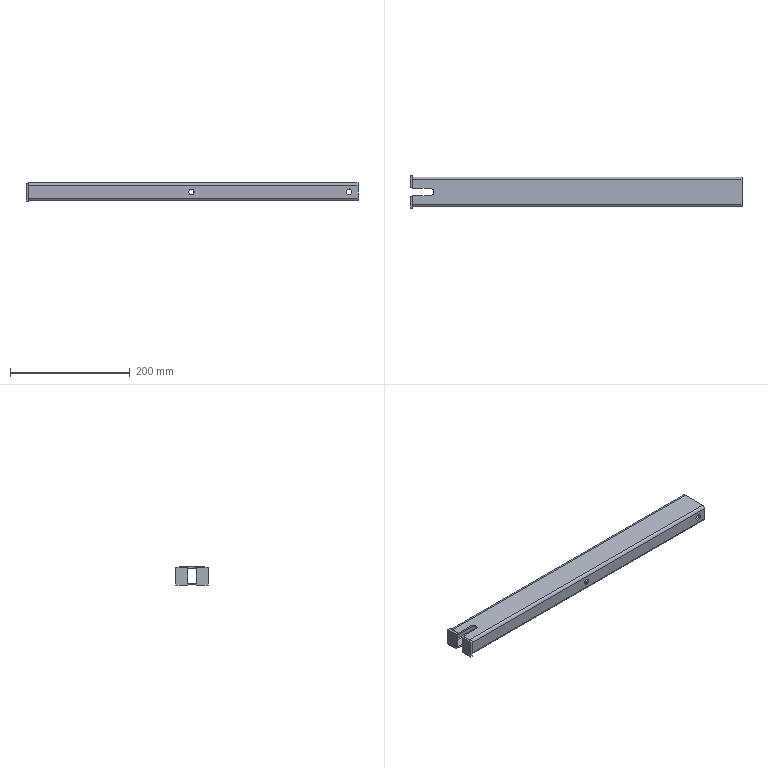Part | SolidWorks | features Cut 2, ICE 2, MirrorSolid 1, WeldMemberFeat 1, WeldmentFeature 1 | 3 solids | 47 faces | box 554 x 54 x 30.061 mm | volume 237150 mm3 | plane 27 | cylinder 20 | commonest cylinder face diameters 9 x8 3 x4 10 x4 12 x4
STEP:
#1=CARTESIAN_POINT('',(39.789,-25.,-4.5));
#2=VERTEX_POINT('',#1);
#3=CARTESIAN_POINT('',(39.789,-25.,4.5));
#4=VERTEX_POINT('',#3);
#5=CARTESIAN_POINT('',(39.789,-25.,0.));
#6=DIRECTION('',(0.,1.,0.));
#7=DIRECTION('',(0.,0.,1.));
#8=AXIS2_PLACEMENT_3D('',#5,#6,#7);
#9=CIRCLE('',#8,4.5);
#10=EDGE_CURVE('',#2,#4,#9,.T.);
#11=ORIENTED_EDGE('',*,*,#10,.F.);
#12=CARTESIAN_POINT('',(39.789,-22.,-4.5));
#13=VERTEX_POINT('',#12);
#14=CARTESIAN_POINT('',(39.789,-25.,-4.5));
#15=DIRECTION('',(0.,1.,0.));
#16=VECTOR('',#15,1000.);
#17=LINE('',#14,#16);
#18=EDGE_CURVE('',#2,#13,#17,.T.);
#19=ORIENTED_EDGE('',*,*,#18,.T.);
#20=CARTESIAN_POINT('',(39.789,-22.,4.5));
#21=VERTEX_POINT('',#20);
#22=CARTESIAN_POINT('',(39.789,-22.,0.));
#23=DIRECTION('',(0.,1.,0.));
#24=DIRECTION('',(0.,0.,1.));
#25=AXIS2_PLACEMENT_3D('',#22,#23,#24);
#26=CIRCLE('',#25,4.5);
#27=EDGE_CURVE('',#13,#21,#26,.T.);
#28=ORIENTED_EDGE('',*,*,#27,.T.);
#29=CARTESIAN_POINT('',(39.789,-25.,4.5));
#30=DIRECTION('',(0.,1.,0.));
#31=VECTOR('',#30,1000.);
#32=LINE('',#29,#31);
#33=EDGE_CURVE('',#4,#21,#32,.T.);
#34=ORIENTED_EDGE('',*,*,#33,.F.);
#35=EDGE_LOOP('',(#11,#19,#28,#34));
#36=FACE_OUTER_BOUND('',#35,.T.);
#37=CARTESIAN_POINT('',(39.789,-25.,0.));
#38=DIRECTION('',(0.,1.,0.));
#39=DIRECTION('',(0.,0.,1.));
#40=AXIS2_PLACEMENT_3D('',#37,#38,#39);
#41=CYLINDRICAL_SURFACE('',#40,4.5);
#42=ADVANCED_FACE('',(#36),#41,.F.);
#43=CARTESIAN_POINT('',(39.789,22.,4.5));
#44=VERTEX_POINT('',#43);
#45=CARTESIAN_POINT('',(39.789,22.,-4.5));
#46=VERTEX_POINT('',#45);
#47=CARTESIAN_POINT('',(39.789,22.,0.));
#48=DIRECTION('',(0.,-1.,0.));
#49=DIRECTION('',(0.,0.,-1.));
#50=AXIS2_PLACEMENT_3D('',#47,#48,#49);
#51=CIRCLE('',#50,4.5);
#52=EDGE_CURVE('',#44,#46,#51,.T.);
#53=ORIENTED_EDGE('',*,*,#52,.T.);
#54=CARTESIAN_POINT('',(39.789,25.,-4.5));
#55=VERTEX_POINT('',#54);
#56=CARTESIAN_POINT('',(39.789,-25.,-4.5));
#57=DIRECTION('',(0.,1.,0.));
#58=VECTOR('',#57,1000.);
#59=LINE('',#56,#58);
#60=EDGE_CURVE('',#46,#55,#59,.T.);
#61=ORIENTED_EDGE('',*,*,#60,.T.);
#62=CARTESIAN_POINT('',(39.789,25.,4.5));
#63=VERTEX_POINT('',#62);
#64=CARTESIAN_POINT('',(39.789,25.,0.));
#65=DIRECTION('',(0.,1.,0.));
#66=DIRECTION('',(0.,0.,1.));
#67=AXIS2_PLACEMENT_3D('',#64,#65,#66);
#68=CIRCLE('',#67,4.5);
#69=EDGE_CURVE('',#55,#63,#68,.T.);
#70=ORIENTED_EDGE('',*,*,#69,.T.);
#71=CARTESIAN_POINT('',(39.789,-25.,4.5));
#72=DIRECTION('',(0.,1.,0.));
#73=VECTOR('',#72,1000.);
#74=LINE('',#71,#73);
#75=EDGE_CURVE('',#44,#63,#74,.T.);
#76=ORIENTED_EDGE('',*,*,#75,.F.);
#77=EDGE_LOOP('',(#53,#61,#70,#76));
#78=FACE_OUTER_BOUND('',#77,.T.);
#79=CARTESIAN_POINT('',(39.789,-25.,0.));
#80=DIRECTION('',(0.,1.,0.));
#81=DIRECTION('',(0.,0.,1.));
#82=AXIS2_PLACEMENT_3D('',#79,#80,#81);
#83=CYLINDRICAL_SURFACE('',#82,4.5);
#84=ADVANCED_FACE('',(#78),#83,.F.);
#85=CARTESIAN_POINT('',(302.789,-22.,-5.));
#86=VERTEX_POINT('',#85);
#87=CARTESIAN_POINT('',(302.789,-22.,5.));
#88=VERTEX_POINT('',#87);
#89=CARTESIAN_POINT('',(302.789,-22.,0.));
#90=DIRECTION('',(0.,1.,0.));
#91=DIRECTION('',(0.,0.,1.));
#92=AXIS2_PLACEMENT_3D('',#89,#90,#91);
#93=CIRCLE('',#92,5.);
#94=EDGE_CURVE('',#86,#88,#93,.T.);
#95=ORIENTED_EDGE('',*,*,#94,.T.);
#96=CARTESIAN_POINT('',(302.789,-25.,5.));
#97=VERTEX_POINT('',#96);
#98=CARTESIAN_POINT('',(302.789,25.,5.));
#99=DIRECTION('',(0.,-1.,0.));
#100=VECTOR('',#99,1000.);
#101=LINE('',#98,#100);
#102=EDGE_CURVE('',#88,#97,#101,.T.);
#103=ORIENTED_EDGE('',*,*,#102,.T.);
#104=CARTESIAN_POINT('',(302.789,-25.,-5.));
#105=VERTEX_POINT('',#104);
#106=CARTESIAN_POINT('',(302.789,-25.,0.));
#107=DIRECTION('',(0.,-1.,0.));
#108=DIRECTION('',(0.,0.,-1.));
#109=AXIS2_PLACEMENT_3D('',#106,#107,#108);
#110=CIRCLE('',#109,5.);
#111=EDGE_CURVE('',#97,#105,#110,.T.);
#112=ORIENTED_EDGE('',*,*,#111,.T.);
#113=CARTESIAN_POINT('',(302.789,25.,-5.));
#114=DIRECTION('',(0.,-1.,0.));
#115=VECTOR('',#114,1000.);
#116=LINE('',#113,#115);
#117=EDGE_CURVE('',#86,#105,#116,.T.);
#118=ORIENTED_EDGE('',*,*,#117,.F.);
#119=EDGE_LOOP('',(#95,#103,#112,#118));
#120=FACE_OUTER_BOUND('',#119,.T.);
#121=CARTESIAN_POINT('',(302.789,25.,0.));
#122=DIRECTION('',(0.,-1.,0.));
#123=DIRECTION('',(0.,0.,-1.));
#124=AXIS2_PLACEMENT_3D('',#121,#122,#123);
#125=CYLINDRICAL_SURFACE('',#124,5.);
#126=ADVANCED_FACE('',(#120),#125,.F.);
#127=CARTESIAN_POINT('',(302.789,25.,5.));
#128=VERTEX_POINT('',#127);
#129=CARTESIAN_POINT('',(302.789,25.,-5.));
#130=VERTEX_POINT('',#129);
#131=CARTESIAN_POINT('',(302.789,25.,0.));
#132=DIRECTION('',(0.,-1.,0.));
#133=DIRECTION('',(0.,0.,-1.));
#134=AXIS2_PLACEMENT_3D('',#131,#132,#133);
#135=CIRCLE('',#134,5.);
#136=EDGE_CURVE('',#128,#130,#135,.T.);
#137=ORIENTED_EDGE('',*,*,#136,.F.);
#138=CARTESIAN_POINT('',(302.789,22.,5.));
#139=VERTEX_POINT('',#138);
#140=CARTESIAN_POINT('',(302.789,25.,5.));
#141=DIRECTION('',(0.,-1.,0.));
#142=VECTOR('',#141,1000.);
#143=LINE('',#140,#142);
#144=EDGE_CURVE('',#128,#139,#143,.T.);
#145=ORIENTED_EDGE('',*,*,#144,.T.);
#146=CARTESIAN_POINT('',(302.789,22.,-5.));
#147=VERTEX_POINT('',#146);
#148=CARTESIAN_POINT('',(302.789,22.,0.));
#149=DIRECTION('',(0.,-1.,0.));
#150=DIRECTION('',(0.,0.,-1.));
#151=AXIS2_PLACEMENT_3D('',#148,#149,#150);
#152=CIRCLE('',#151,5.);
#153=EDGE_CURVE('',#139,#147,#152,.T.);
#154=ORIENTED_EDGE('',*,*,#153,.T.);
#155=CARTESIAN_POINT('',(302.789,25.,-5.));
#156=DIRECTION('',(0.,-1.,0.));
#157=VECTOR('',#156,1000.);
#158=LINE('',#155,#157);
#159=EDGE_CURVE('',#130,#147,#158,.T.);
#160=ORIENTED_EDGE('',*,*,#159,.F.);
#161=EDGE_LOOP('',(#137,#145,#154,#160));
#162=FACE_OUTER_BOUND('',#161,.T.);
#163=CARTESIAN_POINT('',(302.789,25.,0.));
#164=DIRECTION('',(0.,-1.,0.));
#165=DIRECTION('',(0.,0.,-1.));
#166=AXIS2_PLACEMENT_3D('',#163,#164,#165);
#167=CYLINDRICAL_SURFACE('',#166,5.);
#168=ADVANCED_FACE('',(#162),#167,.F.);
#169=CARTESIAN_POINT('',(-202.211,6.,12.));
#170=VERTEX_POINT('',#169);
#171=CARTESIAN_POINT('',(-196.211,0.,12.));
#172=VERTEX_POINT('',#171);
#173=CARTESIAN_POINT('',(-202.211,0.,12.));
#174=DIRECTION('',(0.,0.,-1.));
#175=DIRECTION('',(-1.,0.,0.));
#176=AXIS2_PLACEMENT_3D('',#173,#174,#175);
#177=CIRCLE('',#176,6.);
#178=EDGE_CURVE('',#170,#172,#177,.T.);
#179=ORIENTED_EDGE('',*,*,#178,.T.);
#180=CARTESIAN_POINT('',(-196.211,0.,15.));
#181=VERTEX_POINT('',#180);
#182=CARTESIAN_POINT('',(-196.211,0.,-15.));
#183=DIRECTION('',(0.,0.,1.));
#184=VECTOR('',#183,1000.);
#185=LINE('',#182,#184);
#186=EDGE_CURVE('',#172,#181,#185,.T.);
#187=ORIENTED_EDGE('',*,*,#186,.T.);
#188=CARTESIAN_POINT('',(-202.211,6.,15.));
#189=VERTEX_POINT('',#188);
#190=CARTESIAN_POINT('',(-202.211,0.,15.));
#191=DIRECTION('',(0.,0.,1.));
#192=DIRECTION('',(1.,0.,0.));
#193=AXIS2_PLACEMENT_3D('',#190,#191,#192);
#194=CIRCLE('',#193,6.);
#195=EDGE_CURVE('',#181,#189,#194,.T.);
#196=ORIENTED_EDGE('',*,*,#195,.T.);
#197=CARTESIAN_POINT('',(-202.211,6.,-15.));
#198=DIRECTION('',(0.,0.,1.));
#199=VECTOR('',#198,1000.);
#200=LINE('',#197,#199);
#201=EDGE_CURVE('',#170,#189,#200,.T.);
#202=ORIENTED_EDGE('',*,*,#201,.F.);
#203=EDGE_LOOP('',(#179,#187,#196,#202));
#204=FACE_OUTER_BOUND('',#203,.T.);
#205=CARTESIAN_POINT('',(-202.211,0.,-15.));
#206=DIRECTION('',(0.,0.,1.));
#207=DIRECTION('',(1.,0.,0.));
#208=AXIS2_PLACEMENT_3D('',#205,#206,#207);
#209=CYLINDRICAL_SURFACE('',#208,6.);
#210=ADVANCED_FACE('',(#204),#209,.F.);
#211=CARTESIAN_POINT('',(-196.211,0.,-15.));
#212=VERTEX_POINT('',#211);
#213=CARTESIAN_POINT('',(-202.211,6.,-15.));
#214=VERTEX_POINT('',#213);
#215=CARTESIAN_POINT('',(-202.211,0.,-15.));
#216=DIRECTION('',(0.,0.,1.));
#217=DIRECTION('',(1.,0.,0.));
#218=AXIS2_PLACEMENT_3D('',#215,#216,#217);
#219=CIRCLE('',#218,6.);
#220=EDGE_CURVE('',#212,#214,#219,.T.);
#221=ORIENTED_EDGE('',*,*,#220,.F.);
#222=CARTESIAN_POINT('',(-196.211,0.,-12.));
#223=VERTEX_POINT('',#222);
#224=CARTESIAN_POINT('',(-196.211,0.,-15.));
#225=DIRECTION('',(0.,0.,1.));
#226=VECTOR('',#225,1000.);
#227=LINE('',#224,#226);
#228=EDGE_CURVE('',#212,#223,#227,.T.);
#229=ORIENTED_EDGE('',*,*,#228,.T.);
#230=CARTESIAN_POINT('',(-202.211,6.,-12.));
#231=VERTEX_POINT('',#230);
#232=CARTESIAN_POINT('',(-202.211,0.,-12.));
#233=DIRECTION('',(0.,0.,1.));
#234=DIRECTION('',(1.,0.,0.));
#235=AXIS2_PLACEMENT_3D('',#232,#233,#234);
#236=CIRCLE('',#235,6.);
#237=EDGE_CURVE('',#223,#231,#236,.T.);
#238=ORIENTED_EDGE('',*,*,#237,.T.);
#239=CARTESIAN_POINT('',(-202.211,6.,-15.));
#240=DIRECTION('',(0.,0.,1.));
#241=VECTOR('',#240,1000.);
#242=LINE('',#239,#241);
#243=EDGE_CURVE('',#214,#231,#242,.T.);
#244=ORIENTED_EDGE('',*,*,#243,.F.);
#245=EDGE_LOOP('',(#221,#229,#238,#244));
#246=FACE_OUTER_BOUND('',#245,.T.);
#247=CARTESIAN_POINT('',(-202.211,0.,-15.));
#248=DIRECTION('',(0.,0.,1.));
#249=DIRECTION('',(1.,0.,0.));
#250=AXIS2_PLACEMENT_3D('',#247,#248,#249);
#251=CYLINDRICAL_SURFACE('',#250,6.);
#252=ADVANCED_FACE('',(#246),#251,.F.);
#253=CARTESIAN_POINT('',(-232.211,6.,-15.));
#254=VERTEX_POINT('',#253);
#255=CARTESIAN_POINT('',(-232.211,20.5,-15.));
#256=VERTEX_POINT('',#255);
#257=CARTESIAN_POINT('',(-232.211,-20.5,-15.));
#258=DIRECTION('',(0.,1.,0.));
#259=VECTOR('',#258,1000.);
#260=LINE('',#257,#259);
#261=EDGE_CURVE('',#254,#256,#260,.T.);
#262=ORIENTED_EDGE('',*,*,#261,.F.);
#263=CARTESIAN_POINT('',(-232.211,6.,-12.));
#264=VERTEX_POINT('',#263);
#265=CARTESIAN_POINT('',(-232.211,6.,-15.));
#266=DIRECTION('',(0.,0.,1.));
#267=VECTOR('',#266,1000.);
#268=LINE('',#265,#267);
#269=EDGE_CURVE('',#254,#264,#268,.T.);
#270=ORIENTED_EDGE('',*,*,#269,.T.);
#271=CARTESIAN_POINT('',(-232.211,20.5,-12.));
#272=VERTEX_POINT('',#271);
#273=CARTESIAN_POINT('',(-232.211,-20.5,-12.));
#274=DIRECTION('',(0.,1.,0.));
#275=VECTOR('',#274,1000.);
#276=LINE('',#273,#275);
#277=EDGE_CURVE('',#264,#272,#276,.T.);
#278=ORIENTED_EDGE('',*,*,#277,.T.);
#279=CARTESIAN_POINT('',(-232.211,22.,-10.5));
#280=VERTEX_POINT('',#279);
#281=CARTESIAN_POINT('',(-232.211,20.5,-10.5));
#282=DIRECTION('',(1.,0.,0.));
#283=DIRECTION('',(0.,0.,-1.));
#284=AXIS2_PLACEMENT_3D('',#281,#282,#283);
#285=CIRCLE('',#284,1.5);
#286=EDGE_CURVE('',#272,#280,#285,.T.);
#287=ORIENTED_EDGE('',*,*,#286,.T.);
#288=CARTESIAN_POINT('',(-232.211,22.,10.5));
#289=VERTEX_POINT('',#288);
#290=CARTESIAN_POINT('',(-232.211,22.,10.5));
#291=DIRECTION('',(0.,0.,1.));
#292=VECTOR('',#291,1000.);
#293=LINE('',#290,#292);
#294=EDGE_CURVE('',#280,#289,#293,.T.);
#295=ORIENTED_EDGE('',*,*,#294,.T.);
#296=CARTESIAN_POINT('',(-232.211,20.5,12.));
#297=VERTEX_POINT('',#296);
#298=CARTESIAN_POINT('',(-232.211,20.5,10.5));
#299=DIRECTION('',(1.,0.,0.));
#300=DIRECTION('',(0.,0.,-1.));
#301=AXIS2_PLACEMENT_3D('',#298,#299,#300);
#302=CIRCLE('',#301,1.5);
#303=EDGE_CURVE('',#289,#297,#302,.T.);
#304=ORIENTED_EDGE('',*,*,#303,.T.);
#305=CARTESIAN_POINT('',(-232.211,6.,12.));
#306=VERTEX_POINT('',#305);
#307=CARTESIAN_POINT('',(-232.211,20.5,12.));
#308=DIRECTION('',(0.,-1.,0.));
#309=VECTOR('',#308,1000.);
#310=LINE('',#307,#309);
#311=EDGE_CURVE('',#297,#306,#310,.T.);
#312=ORIENTED_EDGE('',*,*,#311,.T.);
#313=CARTESIAN_POINT('',(-232.211,6.,15.));
#314=VERTEX_POINT('',#313);
#315=CARTESIAN_POINT('',(-232.211,6.,10.5));
#316=DIRECTION('',(0.,0.,1.));
#317=VECTOR('',#316,1000.);
#318=LINE('',#315,#317);
#319=EDGE_CURVE('',#306,#314,#318,.T.);
#320=ORIENTED_EDGE('',*,*,#319,.T.);
#321=CARTESIAN_POINT('',(-232.211,20.5,15.));
#322=VERTEX_POINT('',#321);
#323=CARTESIAN_POINT('',(-232.211,20.5,15.));
#324=DIRECTION('',(0.,-1.,0.));
#325=VECTOR('',#324,1000.);
#326=LINE('',#323,#325);
#327=EDGE_CURVE('',#322,#314,#326,.T.);
#328=ORIENTED_EDGE('',*,*,#327,.F.);
#329=CARTESIAN_POINT('',(-232.211,25.,10.5));
#330=VERTEX_POINT('',#329);
#331=CARTESIAN_POINT('',(-232.211,20.5,10.5));
#332=DIRECTION('',(1.,0.,0.));
#333=DIRECTION('',(0.,0.,-1.));
#334=AXIS2_PLACEMENT_3D('',#331,#332,#333);
#335=CIRCLE('',#334,4.5);
#336=EDGE_CURVE('',#330,#322,#335,.T.);
#337=ORIENTED_EDGE('',*,*,#336,.F.);
#338=CARTESIAN_POINT('',(-232.211,25.,-10.5));
#339=VERTEX_POINT('',#338);
#340=CARTESIAN_POINT('',(-232.211,25.,10.5));
#341=DIRECTION('',(0.,0.,1.));
#342=VECTOR('',#341,1000.);
#343=LINE('',#340,#342);
#344=EDGE_CURVE('',#339,#330,#343,.T.);
#345=ORIENTED_EDGE('',*,*,#344,.F.);
#346=CARTESIAN_POINT('',(-232.211,20.5,-10.5));
#347=DIRECTION('',(1.,0.,0.));
#348=DIRECTION('',(0.,0.,-1.));
#349=AXIS2_PLACEMENT_3D('',#346,#347,#348);
#350=CIRCLE('',#349,4.5);
#351=EDGE_CURVE('',#256,#339,#350,.T.);
#352=ORIENTED_EDGE('',*,*,#351,.F.);
#353=EDGE_LOOP('',(#262,#270,#278,#287,#295,#304,#312,#320,#328,#337,#345,#352));
#354=FACE_OUTER_BOUND('',#353,.T.);
#355=CARTESIAN_POINT('',(-232.211,20.5,10.5));
#356=DIRECTION('',(1.,0.,0.));
#357=DIRECTION('',(0.,0.,-1.));
#358=AXIS2_PLACEMENT_3D('',#355,#356,#357);
#359=PLANE('',#358);
#360=ADVANCED_FACE('',(#354),#359,.F.);
#361=ORIENTED_EDGE('',*,*,#336,.T.);
#362=CARTESIAN_POINT('',(317.789,20.5,15.));
#363=VERTEX_POINT('',#362);
#364=CARTESIAN_POINT('',(317.789,20.5,15.));
#365=DIRECTION('',(-1.,0.,0.));
#366=VECTOR('',#365,1000.);
#367=LINE('',#364,#366);
#368=EDGE_CURVE('',#363,#322,#367,.T.);
#369=ORIENTED_EDGE('',*,*,#368,.F.);
#370=CARTESIAN_POINT('',(317.789,25.,10.5));
#371=VERTEX_POINT('',#370);
#372=CARTESIAN_POINT('',(317.789,20.5,10.5));
#373=DIRECTION('',(1.,0.,0.));
#374=DIRECTION('',(0.,0.,-1.));
#375=AXIS2_PLACEMENT_3D('',#372,#373,#374);
#376=CIRCLE('',#375,4.5);
#377=EDGE_CURVE('',#371,#363,#376,.T.);
#378=ORIENTED_EDGE('',*,*,#377,.F.);
#379=CARTESIAN_POINT('',(317.789,25.,10.5));
#380=DIRECTION('',(-1.,0.,0.));
#381=VECTOR('',#380,1000.);
#382=LINE('',#379,#381);
#383=EDGE_CURVE('',#371,#330,#382,.T.);
#384=ORIENTED_EDGE('',*,*,#383,.T.);
#385=EDGE_LOOP('',(#361,#369,#378,#384));
#386=FACE_OUTER_BOUND('',#385,.T.);
#387=CARTESIAN_POINT('',(317.789,20.5,10.5));
#388=DIRECTION('',(-1.,0.,0.));
#389=DIRECTION('',(0.,0.,1.));
#390=AXIS2_PLACEMENT_3D('',#387,#388,#389);
#391=CYLINDRICAL_SURFACE('',#390,4.5);
#392=ADVANCED_FACE('',(#386),#391,.T.);
#393=ORIENTED_EDGE('',*,*,#327,.T.);
#394=CARTESIAN_POINT('',(-232.211,6.,15.));
#395=DIRECTION('',(-1.,0.,0.));
#396=VECTOR('',#395,1000.);
#397=LINE('',#394,#396);
#398=EDGE_CURVE('',#189,#314,#397,.T.);
#399=ORIENTED_EDGE('',*,*,#398,.F.);
#400=ORIENTED_EDGE('',*,*,#195,.F.);
#401=CARTESIAN_POINT('',(-202.211,-6.,15.));
#402=VERTEX_POINT('',#401);
#403=CARTESIAN_POINT('',(-202.211,0.,15.));
#404=DIRECTION('',(0.,0.,1.));
#405=DIRECTION('',(1.,0.,0.));
#406=AXIS2_PLACEMENT_3D('',#403,#404,#405);
#407=CIRCLE('',#406,6.);
#408=EDGE_CURVE('',#402,#181,#407,.T.);
#409=ORIENTED_EDGE('',*,*,#408,.F.);
#410=CARTESIAN_POINT('',(-232.211,-6.,15.));
#411=VERTEX_POINT('',#410);
#412=CARTESIAN_POINT('',(-232.211,-6.,15.));
#413=DIRECTION('',(1.,0.,0.));
#414=VECTOR('',#413,1000.);
#415=LINE('',#412,#414);
#416=EDGE_CURVE('',#411,#402,#415,.T.);
#417=ORIENTED_EDGE('',*,*,#416,.F.);
#418=CARTESIAN_POINT('',(-232.211,-20.5,15.));
#419=VERTEX_POINT('',#418);
#420=CARTESIAN_POINT('',(-232.211,20.5,15.));
#421=DIRECTION('',(0.,-1.,0.));
#422=VECTOR('',#421,1000.);
#423=LINE('',#420,#422);
#424=EDGE_CURVE('',#411,#419,#423,.T.);
#425=ORIENTED_EDGE('',*,*,#424,.T.);
#426=CARTESIAN_POINT('',(317.789,-20.5,15.));
#427=VERTEX_POINT('',#426);
#428=CARTESIAN_POINT('',(317.789,-20.5,15.));
#429=DIRECTION('',(-1.,0.,0.));
#430=VECTOR('',#429,1000.);
#431=LINE('',#428,#430);
#432=EDGE_CURVE('',#427,#419,#431,.T.);
#433=ORIENTED_EDGE('',*,*,#432,.F.);
#434=CARTESIAN_POINT('',(317.789,20.5,15.));
#435=DIRECTION('',(0.,-1.,0.));
#436=VECTOR('',#435,1000.);
#437=LINE('',#434,#436);
#438=EDGE_CURVE('',#363,#427,#437,.T.);
#439=ORIENTED_EDGE('',*,*,#438,.F.);
#440=ORIENTED_EDGE('',*,*,#368,.T.);
#441=EDGE_LOOP('',(#393,#399,#400,#409,#417,#425,#433,#439,#440));
#442=FACE_OUTER_BOUND('',#441,.T.);
#443=CARTESIAN_POINT('',(317.789,20.5,15.));
#444=DIRECTION('',(0.,0.,-1.));
#445=DIRECTION('',(-1.,0.,0.));
#446=AXIS2_PLACEMENT_3D('',#443,#444,#445);
#447=PLANE('',#446);
#448=ADVANCED_FACE('',(#442),#447,.F.);
#449=CARTESIAN_POINT('',(-232.211,-25.,10.5));
#450=VERTEX_POINT('',#449);
#451=CARTESIAN_POINT('',(-232.211,-20.5,10.5));
#452=DIRECTION('',(1.,0.,0.));
#453=DIRECTION('',(0.,0.,-1.));
#454=AXIS2_PLACEMENT_3D('',#451,#452,#453);
#455=CIRCLE('',#454,4.5);
#456=EDGE_CURVE('',#419,#450,#455,.T.);
#457=ORIENTED_EDGE('',*,*,#456,.T.);
#458=CARTESIAN_POINT('',(317.789,-25.,10.5));
#459=VERTEX_POINT('',#458);
#460=CARTESIAN_POINT('',(317.789,-25.,10.5));
#461=DIRECTION('',(-1.,0.,0.));
#462=VECTOR('',#461,1000.);
#463=LINE('',#460,#462);
#464=EDGE_CURVE('',#459,#450,#463,.T.);
#465=ORIENTED_EDGE('',*,*,#464,.F.);
#466=CARTESIAN_POINT('',(317.789,-20.5,10.5));
#467=DIRECTION('',(1.,0.,0.));
#468=DIRECTION('',(0.,0.,-1.));
#469=AXIS2_PLACEMENT_3D('',#466,#467,#468);
#470=CIRCLE('',#469,4.5);
#471=EDGE_CURVE('',#427,#459,#470,.T.);
#472=ORIENTED_EDGE('',*,*,#471,.F.);
#473=ORIENTED_EDGE('',*,*,#432,.T.);
#474=EDGE_LOOP('',(#457,#465,#472,#473));
#475=FACE_OUTER_BOUND('',#474,.T.);
#476=CARTESIAN_POINT('',(317.789,-20.5,10.5));
#477=DIRECTION('',(-1.,0.,0.));
#478=DIRECTION('',(0.,0.,1.));
#479=AXIS2_PLACEMENT_3D('',#476,#477,#478);
#480=CYLINDRICAL_SURFACE('',#479,4.5);
#481=ADVANCED_FACE('',(#475),#480,.T.);
#482=CARTESIAN_POINT('',(39.789,-25.,0.));
#483=DIRECTION('',(0.,1.,0.));
#484=DIRECTION('',(0.,0.,1.));
#485=AXIS2_PLACEMENT_3D('',#482,#483,#484);
#486=CIRCLE('',#485,4.5);
#487=EDGE_CURVE('',#4,#2,#486,.T.);
#488=ORIENTED_EDGE('',*,*,#487,.T.);
#489=ORIENTED_EDGE('',*,*,#10,.T.);
#490=EDGE_LOOP('',(#488,#489));
#491=FACE_BOUND('',#490,.T.);
#492=CARTESIAN_POINT('',(302.789,-25.,0.));
#493=DIRECTION('',(0.,-1.,0.));
#494=DIRECTION('',(0.,0.,-1.));
#495=AXIS2_PLACEMENT_3D('',#492,#493,#494);
#496=CIRCLE('',#495,5.);
#497=EDGE_CURVE('',#105,#97,#496,.T.);
#498=ORIENTED_EDGE('',*,*,#497,.F.);
#499=ORIENTED_EDGE('',*,*,#111,.F.);
#500=EDGE_LOOP('',(#498,#499));
#501=FACE_BOUND('',#500,.T.);
#502=CARTESIAN_POINT('',(-232.211,-25.,-10.5));
#503=VERTEX_POINT('',#502);
#504=CARTESIAN_POINT('',(-232.211,-25.,-10.5));
#505=DIRECTION('',(0.,0.,-1.));
#506=VECTOR('',#505,1000.);
#507=LINE('',#504,#506);
#508=EDGE_CURVE('',#450,#503,#507,.T.);
#509=ORIENTED_EDGE('',*,*,#508,.T.);
#510=CARTESIAN_POINT('',(317.789,-25.,-10.5));
#511=VERTEX_POINT('',#510);
#512=CARTESIAN_POINT('',(317.789,-25.,-10.5));
#513=DIRECTION('',(-1.,0.,0.));
#514=VECTOR('',#513,1000.);
#515=LINE('',#512,#514);
#516=EDGE_CURVE('',#511,#503,#515,.T.);
#517=ORIENTED_EDGE('',*,*,#516,.F.);
#518=CARTESIAN_POINT('',(317.789,-25.,-10.5));
#519=DIRECTION('',(0.,0.,-1.));
#520=VECTOR('',#519,1000.);
#521=LINE('',#518,#520);
#522=EDGE_CURVE('',#459,#511,#521,.T.);
#523=ORIENTED_EDGE('',*,*,#522,.F.);
#524=ORIENTED_EDGE('',*,*,#464,.T.);
#525=EDGE_LOOP('',(#509,#517,#523,#524));
#526=FACE_OUTER_BOUND('',#525,.T.);
#527=CARTESIAN_POINT('',(317.789,-25.,-10.5));
#528=DIRECTION('',(0.,1.,0.));
#529=DIRECTION('',(0.,0.,1.));
#530=AXIS2_PLACEMENT_3D('',#527,#528,#529);
#531=PLANE('',#530);
#532=ADVANCED_FACE('',(#491,#501,#526),#531,.F.);
#533=CARTESIAN_POINT('',(-232.211,-20.5,-15.));
#534=VERTEX_POINT('',#533);
#535=CARTESIAN_POINT('',(-232.211,-20.5,-10.5));
#536=DIRECTION('',(1.,0.,0.));
#537=DIRECTION('',(0.,0.,-1.));
#538=AXIS2_PLACEMENT_3D('',#535,#536,#537);
#539=CIRCLE('',#538,4.5);
#540=EDGE_CURVE('',#503,#534,#539,.T.);
#541=ORIENTED_EDGE('',*,*,#540,.T.);
#542=CARTESIAN_POINT('',(317.789,-20.5,-15.));
#543=VERTEX_POINT('',#542);
#544=CARTESIAN_POINT('',(317.789,-20.5,-15.));
#545=DIRECTION('',(-1.,0.,0.));
#546=VECTOR('',#545,1000.);
#547=LINE('',#544,#546);
#548=EDGE_CURVE('',#543,#534,#547,.T.);
#549=ORIENTED_EDGE('',*,*,#548,.F.);
#550=CARTESIAN_POINT('',(317.789,-20.5,-10.5));
#551=DIRECTION('',(1.,0.,0.));
#552=DIRECTION('',(0.,0.,-1.));
#553=AXIS2_PLACEMENT_3D('',#550,#551,#552);
#554=CIRCLE('',#553,4.5);
#555=EDGE_CURVE('',#511,#543,#554,.T.);
#556=ORIENTED_EDGE('',*,*,#555,.F.);
#557=ORIENTED_EDGE('',*,*,#516,.T.);
#558=EDGE_LOOP('',(#541,#549,#556,#557));
#559=FACE_OUTER_BOUND('',#558,.T.);
#560=CARTESIAN_POINT('',(317.789,-20.5,-10.5));
#561=DIRECTION('',(-1.,0.,0.));
#562=DIRECTION('',(0.,0.,1.));
#563=AXIS2_PLACEMENT_3D('',#560,#561,#562);
#564=CYLINDRICAL_SURFACE('',#563,4.5);
#565=ADVANCED_FACE('',(#559),#564,.T.);
#566=CARTESIAN_POINT('',(-202.211,-6.,-15.));
#567=VERTEX_POINT('',#566);
#568=CARTESIAN_POINT('',(-202.211,0.,-15.));
#569=DIRECTION('',(0.,0.,1.));
#570=DIRECTION('',(1.,0.,0.));
#571=AXIS2_PLACEMENT_3D('',#568,#569,#570);
#572=CIRCLE('',#571,6.);
#573=EDGE_CURVE('',#567,#212,#572,.T.);
#574=ORIENTED_EDGE('',*,*,#573,.T.);
#575=ORIENTED_EDGE('',*,*,#220,.T.);
#576=CARTESIAN_POINT('',(-232.211,6.,-15.));
#577=DIRECTION('',(-1.,0.,0.));
#578=VECTOR('',#577,1000.);
#579=LINE('',#576,#578);
#580=EDGE_CURVE('',#214,#254,#579,.T.);
#581=ORIENTED_EDGE('',*,*,#580,.T.);
#582=ORIENTED_EDGE('',*,*,#261,.T.);
#583=CARTESIAN_POINT('',(317.789,20.5,-15.));
#584=VERTEX_POINT('',#583);
#585=CARTESIAN_POINT('',(317.789,20.5,-15.));
#586=DIRECTION('',(-1.,0.,0.));
#587=VECTOR('',#586,1000.);
#588=LINE('',#585,#587);
#589=EDGE_CURVE('',#584,#256,#588,.T.);
#590=ORIENTED_EDGE('',*,*,#589,.F.);
#591=CARTESIAN_POINT('',(317.789,-20.5,-15.));
#592=DIRECTION('',(0.,1.,0.));
#593=VECTOR('',#592,1000.);
#594=LINE('',#591,#593);
#595=EDGE_CURVE('',#543,#584,#594,.T.);
#596=ORIENTED_EDGE('',*,*,#595,.F.);
#597=ORIENTED_EDGE('',*,*,#548,.T.);
#598=CARTESIAN_POINT('',(-232.211,-6.,-15.));
#599=VERTEX_POINT('',#598);
#600=CARTESIAN_POINT('',(-232.211,-20.5,-15.));
#601=DIRECTION('',(0.,1.,0.));
#602=VECTOR('',#601,1000.);
#603=LINE('',#600,#602);
#604=EDGE_CURVE('',#534,#599,#603,.T.);
#605=ORIENTED_EDGE('',*,*,#604,.T.);
#606=CARTESIAN_POINT('',(-232.211,-6.,-15.));
#607=DIRECTION('',(1.,0.,0.));
#608=VECTOR('',#607,1000.);
#609=LINE('',#606,#608);
#610=EDGE_CURVE('',#599,#567,#609,.T.);
#611=ORIENTED_EDGE('',*,*,#610,.T.);
#612=EDGE_LOOP('',(#574,#575,#581,#582,#590,#596,#597,#605,#611));
#613=FACE_OUTER_BOUND('',#612,.T.);
#614=CARTESIAN_POINT('',(317.789,-20.5,-15.));
#615=DIRECTION('',(0.,0.,1.));
#616=DIRECTION('',(1.,0.,0.));
#617=AXIS2_PLACEMENT_3D('',#614,#615,#616);
#618=PLANE('',#617);
#619=ADVANCED_FACE('',(#613),#618,.F.);
#620=ORIENTED_EDGE('',*,*,#351,.T.);
#621=CARTESIAN_POINT('',(317.789,25.,-10.5));
#622=VERTEX_POINT('',#621);
#623=CARTESIAN_POINT('',(317.789,25.,-10.5));
#624=DIRECTION('',(-1.,0.,0.));
#625=VECTOR('',#624,1000.);
#626=LINE('',#623,#625);
#627=EDGE_CURVE('',#622,#339,#626,.T.);
#628=ORIENTED_EDGE('',*,*,#627,.F.);
#629=CARTESIAN_POINT('',(317.789,20.5,-10.5));
#630=DIRECTION('',(1.,0.,0.));
#631=DIRECTION('',(0.,0.,-1.));
#632=AXIS2_PLACEMENT_3D('',#629,#630,#631);
#633=CIRCLE('',#632,4.5);
#634=EDGE_CURVE('',#584,#622,#633,.T.);
#635=ORIENTED_EDGE('',*,*,#634,.F.);
#636=ORIENTED_EDGE('',*,*,#589,.T.);
#637=EDGE_LOOP('',(#620,#628,#635,#636));
#638=FACE_OUTER_BOUND('',#637,.T.);
#639=CARTESIAN_POINT('',(317.789,20.5,-10.5));
#640=DIRECTION('',(-1.,0.,0.));
#641=DIRECTION('',(0.,0.,1.));
#642=AXIS2_PLACEMENT_3D('',#639,#640,#641);
#643=CYLINDRICAL_SURFACE('',#642,4.5);
#644=ADVANCED_FACE('',(#638),#643,.T.);
#645=CARTESIAN_POINT('',(-232.211,-20.5,12.));
#646=VERTEX_POINT('',#645);
#647=CARTESIAN_POINT('',(-232.211,-22.,10.5));
#648=VERTEX_POINT('',#647);
#649=CARTESIAN_POINT('',(-232.211,-20.5,10.5));
#650=DIRECTION('',(1.,0.,0.));
#651=DIRECTION('',(0.,0.,-1.));
#652=AXIS2_PLACEMENT_3D('',#649,#650,#651);
#653=CIRCLE('',#652,1.5);
#654=EDGE_CURVE('',#646,#648,#653,.T.);
#655=ORIENTED_EDGE('',*,*,#654,.F.);
#656=CARTESIAN_POINT('',(317.789,-20.5,12.));
#657=VERTEX_POINT('',#656);
#658=CARTESIAN_POINT('',(317.789,-20.5,12.));
#659=DIRECTION('',(-1.,0.,0.));
#660=VECTOR('',#659,1000.);
#661=LINE('',#658,#660);
#662=EDGE_CURVE('',#657,#646,#661,.T.);
#663=ORIENTED_EDGE('',*,*,#662,.F.);
#664=CARTESIAN_POINT('',(317.789,-22.,10.5));
#665=VERTEX_POINT('',#664);
#666=CARTESIAN_POINT('',(317.789,-20.5,10.5));
#667=DIRECTION('',(1.,0.,0.));
#668=DIRECTION('',(0.,0.,-1.));
#669=AXIS2_PLACEMENT_3D('',#666,#667,#668);
#670=CIRCLE('',#669,1.5);
#671=EDGE_CURVE('',#657,#665,#670,.T.);
#672=ORIENTED_EDGE('',*,*,#671,.T.);
#673=CARTESIAN_POINT('',(317.789,-22.,10.5));
#674=DIRECTION('',(-1.,0.,0.));
#675=VECTOR('',#674,1000.);
#676=LINE('',#673,#675);
#677=EDGE_CURVE('',#665,#648,#676,.T.);
#678=ORIENTED_EDGE('',*,*,#677,.T.);
#679=EDGE_LOOP('',(#655,#663,#672,#678));
#680=FACE_OUTER_BOUND('',#679,.T.);
#681=CARTESIAN_POINT('',(317.789,-20.5,10.5));
#682=DIRECTION('',(-1.,0.,0.));
#683=DIRECTION('',(0.,0.,1.));
#684=AXIS2_PLACEMENT_3D('',#681,#682,#683);
#685=CYLINDRICAL_SURFACE('',#684,1.5);
#686=ADVANCED_FACE('',(#680),#685,.F.);
#687=CARTESIAN_POINT('',(317.789,6.,12.));
#688=DIRECTION('',(1.,0.,0.));
#689=VECTOR('',#688,1000.);
#690=LINE('',#687,#689);
#691=EDGE_CURVE('',#306,#170,#690,.T.);
#692=ORIENTED_EDGE('',*,*,#691,.F.);
#693=ORIENTED_EDGE('',*,*,#311,.F.);
#694=CARTESIAN_POINT('',(317.789,20.5,12.));
#695=VERTEX_POINT('',#694);
#696=CARTESIAN_POINT('',(317.789,20.5,12.));
#697=DIRECTION('',(-1.,0.,0.));
#698=VECTOR('',#697,1000.);
#699=LINE('',#696,#698);
#700=EDGE_CURVE('',#695,#297,#699,.T.);
#701=ORIENTED_EDGE('',*,*,#700,.F.);
#702=CARTESIAN_POINT('',(317.789,20.5,12.));
#703=DIRECTION('',(0.,-1.,0.));
#704=VECTOR('',#703,1000.);
#705=LINE('',#702,#704);
#706=EDGE_CURVE('',#695,#657,#705,.T.);
#707=ORIENTED_EDGE('',*,*,#706,.T.);
#708=ORIENTED_EDGE('',*,*,#662,.T.);
#709=CARTESIAN_POINT('',(-232.211,-6.,12.));
#710=VERTEX_POINT('',#709);
#711=CARTESIAN_POINT('',(-232.211,20.5,12.));
#712=DIRECTION('',(0.,-1.,0.));
#713=VECTOR('',#712,1000.);
#714=LINE('',#711,#713);
#715=EDGE_CURVE('',#710,#646,#714,.T.);
#716=ORIENTED_EDGE('',*,*,#715,.F.);
#717=CARTESIAN_POINT('',(-202.211,-6.,12.));
#718=VERTEX_POINT('',#717);
#719=CARTESIAN_POINT('',(317.789,-6.,12.));
#720=DIRECTION('',(-1.,0.,0.));
#721=VECTOR('',#720,1000.);
#722=LINE('',#719,#721);
#723=EDGE_CURVE('',#718,#710,#722,.T.);
#724=ORIENTED_EDGE('',*,*,#723,.F.);
#725=CARTESIAN_POINT('',(-202.211,0.,12.));
#726=DIRECTION('',(0.,0.,-1.));
#727=DIRECTION('',(-1.,0.,0.));
#728=AXIS2_PLACEMENT_3D('',#725,#726,#727);
#729=CIRCLE('',#728,6.);
#730=EDGE_CURVE('',#172,#718,#729,.T.);
#731=ORIENTED_EDGE('',*,*,#730,.F.);
#732=ORIENTED_EDGE('',*,*,#178,.F.);
#733=EDGE_LOOP('',(#692,#693,#701,#707,#708,#716,#724,#731,#732));
#734=FACE_OUTER_BOUND('',#733,.T.);
#735=CARTESIAN_POINT('',(317.789,20.5,12.));
#736=DIRECTION('',(0.,0.,-1.));
#737=DIRECTION('',(-1.,0.,0.));
#738=AXIS2_PLACEMENT_3D('',#735,#736,#737);
#739=PLANE('',#738);
#740=ADVANCED_FACE('',(#734),#739,.T.);
#741=ORIENTED_EDGE('',*,*,#303,.F.);
#742=CARTESIAN_POINT('',(317.789,22.,10.5));
#743=VERTEX_POINT('',#742);
#744=CARTESIAN_POINT('',(317.789,22.,10.5));
#745=DIRECTION('',(-1.,0.,0.));
#746=VECTOR('',#745,1000.);
#747=LINE('',#744,#746);
#748=EDGE_CURVE('',#743,#289,#747,.T.);
#749=ORIENTED_EDGE('',*,*,#748,.F.);
#750=CARTESIAN_POINT('',(317.789,20.5,10.5));
#751=DIRECTION('',(1.,0.,0.));
#752=DIRECTION('',(0.,0.,-1.));
#753=AXIS2_PLACEMENT_3D('',#750,#751,#752);
#754=CIRCLE('',#753,1.5);
#755=EDGE_CURVE('',#743,#695,#754,.T.);
#756=ORIENTED_EDGE('',*,*,#755,.T.);
#757=ORIENTED_EDGE('',*,*,#700,.T.);
#758=EDGE_LOOP('',(#741,#749,#756,#757));
#759=FACE_OUTER_BOUND('',#758,.T.);
#760=CARTESIAN_POINT('',(317.789,20.5,10.5));
#761=DIRECTION('',(-1.,0.,0.));
#762=DIRECTION('',(0.,0.,1.));
#763=AXIS2_PLACEMENT_3D('',#760,#761,#762);
#764=CYLINDRICAL_SURFACE('',#763,1.5);
#765=ADVANCED_FACE('',(#759),#764,.F.);
#766=ORIENTED_EDGE('',*,*,#52,.F.);
#767=CARTESIAN_POINT('',(39.789,22.,0.));
#768=DIRECTION('',(0.,-1.,0.));
#769=DIRECTION('',(0.,0.,-1.));
#770=AXIS2_PLACEMENT_3D('',#767,#768,#769);
#771=CIRCLE('',#770,4.5);
#772=EDGE_CURVE('',#46,#44,#771,.T.);
#773=ORIENTED_EDGE('',*,*,#772,.F.);
#774=EDGE_LOOP('',(#766,#773));
#775=FACE_BOUND('',#774,.T.);
#776=CARTESIAN_POINT('',(302.789,22.,0.));
#777=DIRECTION('',(0.,-1.,0.));
#778=DIRECTION('',(0.,0.,-1.));
#779=AXIS2_PLACEMENT_3D('',#776,#777,#778);
#780=CIRCLE('',#779,5.);
#781=EDGE_CURVE('',#147,#139,#780,.T.);
#782=ORIENTED_EDGE('',*,*,#781,.F.);
#783=ORIENTED_EDGE('',*,*,#153,.F.);
#784=EDGE_LOOP('',(#782,#783));
#785=FACE_BOUND('',#784,.T.);
#786=ORIENTED_EDGE('',*,*,#294,.F.);
#787=CARTESIAN_POINT('',(317.789,22.,-10.5));
#788=VERTEX_POINT('',#787);
#789=CARTESIAN_POINT('',(317.789,22.,-10.5));
#790=DIRECTION('',(-1.,0.,0.));
#791=VECTOR('',#790,1000.);
#792=LINE('',#789,#791);
#793=EDGE_CURVE('',#788,#280,#792,.T.);
#794=ORIENTED_EDGE('',*,*,#793,.F.);
#795=CARTESIAN_POINT('',(317.789,22.,10.5));
#796=DIRECTION('',(0.,0.,1.));
#797=VECTOR('',#796,1000.);
#798=LINE('',#795,#797);
#799=EDGE_CURVE('',#788,#743,#798,.T.);
#800=ORIENTED_EDGE('',*,*,#799,.T.);
#801=ORIENTED_EDGE('',*,*,#748,.T.);
#802=EDGE_LOOP('',(#786,#794,#800,#801));
#803=FACE_OUTER_BOUND('',#802,.T.);
#804=CARTESIAN_POINT('',(317.789,22.,10.5));
#805=DIRECTION('',(0.,-1.,0.));
#806=DIRECTION('',(0.,0.,-1.));
#807=AXIS2_PLACEMENT_3D('',#804,#805,#806);
#808=PLANE('',#807);
#809=ADVANCED_FACE('',(#775,#785,#803),#808,.T.);
#810=ORIENTED_EDGE('',*,*,#286,.F.);
#811=CARTESIAN_POINT('',(317.789,20.5,-12.));
#812=VERTEX_POINT('',#811);
#813=CARTESIAN_POINT('',(317.789,20.5,-12.));
#814=DIRECTION('',(-1.,0.,0.));
#815=VECTOR('',#814,1000.);
#816=LINE('',#813,#815);
#817=EDGE_CURVE('',#812,#272,#816,.T.);
#818=ORIENTED_EDGE('',*,*,#817,.F.);
#819=CARTESIAN_POINT('',(317.789,20.5,-10.5));
#820=DIRECTION('',(1.,0.,0.));
#821=DIRECTION('',(0.,0.,-1.));
#822=AXIS2_PLACEMENT_3D('',#819,#820,#821);
#823=CIRCLE('',#822,1.5);
#824=EDGE_CURVE('',#812,#788,#823,.T.);
#825=ORIENTED_EDGE('',*,*,#824,.T.);
#826=ORIENTED_EDGE('',*,*,#793,.T.);
#827=EDGE_LOOP('',(#810,#818,#825,#826));
#828=FACE_OUTER_BOUND('',#827,.T.);
#829=CARTESIAN_POINT('',(317.789,20.5,-10.5));
#830=DIRECTION('',(-1.,0.,0.));
#831=DIRECTION('',(0.,0.,1.));
#832=AXIS2_PLACEMENT_3D('',#829,#830,#831);
#833=CYLINDRICAL_SURFACE('',#832,1.5);
#834=ADVANCED_FACE('',(#828),#833,.F.);
#835=CARTESIAN_POINT('',(317.789,6.,-12.));
#836=DIRECTION('',(-1.,0.,0.));
#837=VECTOR('',#836,1000.);
#838=LINE('',#835,#837);
#839=EDGE_CURVE('',#231,#264,#838,.T.);
#840=ORIENTED_EDGE('',*,*,#839,.F.);
#841=ORIENTED_EDGE('',*,*,#237,.F.);
#842=CARTESIAN_POINT('',(-202.211,-6.,-12.));
#843=VERTEX_POINT('',#842);
#844=CARTESIAN_POINT('',(-202.211,0.,-12.));
#845=DIRECTION('',(0.,0.,1.));
#846=DIRECTION('',(1.,0.,0.));
#847=AXIS2_PLACEMENT_3D('',#844,#845,#846);
#848=CIRCLE('',#847,6.);
#849=EDGE_CURVE('',#843,#223,#848,.T.);
#850=ORIENTED_EDGE('',*,*,#849,.F.);
#851=CARTESIAN_POINT('',(-232.211,-6.,-12.));
#852=VERTEX_POINT('',#851);
#853=CARTESIAN_POINT('',(317.789,-6.,-12.));
#854=DIRECTION('',(1.,0.,0.));
#855=VECTOR('',#854,1000.);
#856=LINE('',#853,#855);
#857=EDGE_CURVE('',#852,#843,#856,.T.);
#858=ORIENTED_EDGE('',*,*,#857,.F.);
#859=CARTESIAN_POINT('',(-232.211,-20.5,-12.));
#860=VERTEX_POINT('',#859);
#861=CARTESIAN_POINT('',(-232.211,-20.5,-12.));
#862=DIRECTION('',(0.,1.,0.));
#863=VECTOR('',#862,1000.);
#864=LINE('',#861,#863);
#865=EDGE_CURVE('',#860,#852,#864,.T.);
#866=ORIENTED_EDGE('',*,*,#865,.F.);
#867=CARTESIAN_POINT('',(317.789,-20.5,-12.));
#868=VERTEX_POINT('',#867);
#869=CARTESIAN_POINT('',(317.789,-20.5,-12.));
#870=DIRECTION('',(-1.,0.,0.));
#871=VECTOR('',#870,1000.);
#872=LINE('',#869,#871);
#873=EDGE_CURVE('',#868,#860,#872,.T.);
#874=ORIENTED_EDGE('',*,*,#873,.F.);
#875=CARTESIAN_POINT('',(317.789,-20.5,-12.));
#876=DIRECTION('',(0.,1.,0.));
#877=VECTOR('',#876,1000.);
#878=LINE('',#875,#877);
#879=EDGE_CURVE('',#868,#812,#878,.T.);
#880=ORIENTED_EDGE('',*,*,#879,.T.);
#881=ORIENTED_EDGE('',*,*,#817,.T.);
#882=ORIENTED_EDGE('',*,*,#277,.F.);
#883=EDGE_LOOP('',(#840,#841,#850,#858,#866,#874,#880,#881,#882));
#884=FACE_OUTER_BOUND('',#883,.T.);
#885=CARTESIAN_POINT('',(317.789,-20.5,-12.));
#886=DIRECTION('',(0.,0.,1.));
#887=DIRECTION('',(1.,0.,0.));
#888=AXIS2_PLACEMENT_3D('',#885,#886,#887);
#889=PLANE('',#888);
#890=ADVANCED_FACE('',(#884),#889,.T.);
#891=CARTESIAN_POINT('',(-232.211,-22.,-10.5));
#892=VERTEX_POINT('',#891);
#893=CARTESIAN_POINT('',(-232.211,-20.5,-10.5));
#894=DIRECTION('',(1.,0.,0.));
#895=DIRECTION('',(0.,0.,-1.));
#896=AXIS2_PLACEMENT_3D('',#893,#894,#895);
#897=CIRCLE('',#896,1.5);
#898=EDGE_CURVE('',#892,#860,#897,.T.);
#899=ORIENTED_EDGE('',*,*,#898,.F.);
#900=CARTESIAN_POINT('',(317.789,-22.,-10.5));
#901=VERTEX_POINT('',#900);
#902=CARTESIAN_POINT('',(317.789,-22.,-10.5));
#903=DIRECTION('',(-1.,0.,0.));
#904=VECTOR('',#903,1000.);
#905=LINE('',#902,#904);
#906=EDGE_CURVE('',#901,#892,#905,.T.);
#907=ORIENTED_EDGE('',*,*,#906,.F.);
#908=CARTESIAN_POINT('',(317.789,-20.5,-10.5));
#909=DIRECTION('',(1.,0.,0.));
#910=DIRECTION('',(0.,0.,-1.));
#911=AXIS2_PLACEMENT_3D('',#908,#909,#910);
#912=CIRCLE('',#911,1.5);
#913=EDGE_CURVE('',#901,#868,#912,.T.);
#914=ORIENTED_EDGE('',*,*,#913,.T.);
#915=ORIENTED_EDGE('',*,*,#873,.T.);
#916=EDGE_LOOP('',(#899,#907,#914,#915));
#917=FACE_OUTER_BOUND('',#916,.T.);
#918=CARTESIAN_POINT('',(317.789,-20.5,-10.5));
#919=DIRECTION('',(-1.,0.,0.));
#920=DIRECTION('',(0.,0.,1.));
#921=AXIS2_PLACEMENT_3D('',#918,#919,#920);
#922=CYLINDRICAL_SURFACE('',#921,1.5);
#923=ADVANCED_FACE('',(#917),#922,.F.);
#924=CARTESIAN_POINT('',(39.789,-22.,0.));
#925=DIRECTION('',(0.,1.,0.));
#926=DIRECTION('',(0.,0.,1.));
#927=AXIS2_PLACEMENT_3D('',#924,#925,#926);
#928=CIRCLE('',#927,4.5);
#929=EDGE_CURVE('',#21,#13,#928,.T.);
#930=ORIENTED_EDGE('',*,*,#929,.F.);
#931=ORIENTED_EDGE('',*,*,#27,.F.);
#932=EDGE_LOOP('',(#930,#931));
#933=FACE_BOUND('',#932,.T.);
#934=ORIENTED_EDGE('',*,*,#94,.F.);
#935=CARTESIAN_POINT('',(302.789,-22.,0.));
#936=DIRECTION('',(0.,1.,0.));
#937=DIRECTION('',(0.,0.,1.));
#938=AXIS2_PLACEMENT_3D('',#935,#936,#937);
#939=CIRCLE('',#938,5.);
#940=EDGE_CURVE('',#88,#86,#939,.T.);
#941=ORIENTED_EDGE('',*,*,#940,.F.);
#942=EDGE_LOOP('',(#934,#941));
#943=FACE_BOUND('',#942,.T.);
#944=CARTESIAN_POINT('',(-232.211,-22.,-10.5));
#945=DIRECTION('',(0.,0.,-1.));
#946=VECTOR('',#945,1000.);
#947=LINE('',#944,#946);
#948=EDGE_CURVE('',#648,#892,#947,.T.);
#949=ORIENTED_EDGE('',*,*,#948,.F.);
#950=ORIENTED_EDGE('',*,*,#677,.F.);
#951=CARTESIAN_POINT('',(317.789,-22.,-10.5));
#952=DIRECTION('',(0.,0.,-1.));
#953=VECTOR('',#952,1000.);
#954=LINE('',#951,#953);
#955=EDGE_CURVE('',#665,#901,#954,.T.);
#956=ORIENTED_EDGE('',*,*,#955,.T.);
#957=ORIENTED_EDGE('',*,*,#906,.T.);
#958=EDGE_LOOP('',(#949,#950,#956,#957));
#959=FACE_OUTER_BOUND('',#958,.T.);
#960=CARTESIAN_POINT('',(317.789,-22.,-10.5));
#961=DIRECTION('',(0.,1.,0.));
#962=DIRECTION('',(0.,0.,1.));
#963=AXIS2_PLACEMENT_3D('',#960,#961,#962);
#964=PLANE('',#963);
#965=ADVANCED_FACE('',(#933,#943,#959),#964,.T.);
#966=CARTESIAN_POINT('',(39.789,25.,0.));
#967=DIRECTION('',(0.,1.,0.));
#968=DIRECTION('',(0.,0.,1.));
#969=AXIS2_PLACEMENT_3D('',#966,#967,#968);
#970=CIRCLE('',#969,4.5);
#971=EDGE_CURVE('',#63,#55,#970,.T.);
#972=ORIENTED_EDGE('',*,*,#971,.F.);
#973=ORIENTED_EDGE('',*,*,#69,.F.);
#974=EDGE_LOOP('',(#972,#973));
#975=FACE_BOUND('',#974,.T.);
#976=CARTESIAN_POINT('',(302.789,25.,0.));
#977=DIRECTION('',(0.,-1.,0.));
#978=DIRECTION('',(0.,0.,-1.));
#979=AXIS2_PLACEMENT_3D('',#976,#977,#978);
#980=CIRCLE('',#979,5.);
#981=EDGE_CURVE('',#130,#128,#980,.T.);
#982=ORIENTED_EDGE('',*,*,#981,.T.);
#983=ORIENTED_EDGE('',*,*,#136,.T.);
#984=EDGE_LOOP('',(#982,#983));
#985=FACE_BOUND('',#984,.T.);
#986=ORIENTED_EDGE('',*,*,#344,.T.);
#987=ORIENTED_EDGE('',*,*,#383,.F.);
#988=CARTESIAN_POINT('',(317.789,25.,10.5));
#989=DIRECTION('',(0.,0.,1.));
#990=VECTOR('',#989,1000.);
#991=LINE('',#988,#990);
#992=EDGE_CURVE('',#622,#371,#991,.T.);
#993=ORIENTED_EDGE('',*,*,#992,.F.);
#994=ORIENTED_EDGE('',*,*,#627,.T.);
#995=EDGE_LOOP('',(#986,#987,#993,#994));
#996=FACE_OUTER_BOUND('',#995,.T.);
#997=CARTESIAN_POINT('',(317.789,25.,10.5));
#998=DIRECTION('',(0.,-1.,0.));
#999=DIRECTION('',(0.,0.,-1.));
#1000=AXIS2_PLACEMENT_3D('',#997,#998,#999);
#1001=PLANE('',#1000);
#1002=ADVANCED_FACE('',(#975,#985,#996),#1001,.F.);
#1003=ORIENTED_EDGE('',*,*,#671,.F.);
#1004=ORIENTED_EDGE('',*,*,#706,.F.);
#1005=ORIENTED_EDGE('',*,*,#755,.F.);
#1006=ORIENTED_EDGE('',*,*,#799,.F.);
#1007=ORIENTED_EDGE('',*,*,#824,.F.);
#1008=ORIENTED_EDGE('',*,*,#879,.F.);
#1009=ORIENTED_EDGE('',*,*,#913,.F.);
#1010=ORIENTED_EDGE('',*,*,#955,.F.);
#1011=EDGE_LOOP('',(#1003,#1004,#1005,#1006,#1007,#1008,#1009,#1010));
#1012=FACE_BOUND('',#1011,.T.);
#1013=ORIENTED_EDGE('',*,*,#377,.T.);
#1014=ORIENTED_EDGE('',*,*,#438,.T.);
#1015=ORIENTED_EDGE('',*,*,#471,.T.);
#1016=ORIENTED_EDGE('',*,*,#522,.T.);
#1017=ORIENTED_EDGE('',*,*,#555,.T.);
#1018=ORIENTED_EDGE('',*,*,#595,.T.);
#1019=ORIENTED_EDGE('',*,*,#634,.T.);
#1020=ORIENTED_EDGE('',*,*,#992,.T.);
#1021=EDGE_LOOP('',(#1013,#1014,#1015,#1016,#1017,#1018,#1019,#1020));
#1022=FACE_OUTER_BOUND('',#1021,.T.);
#1023=CARTESIAN_POINT('',(317.789,20.5,10.5));
#1024=DIRECTION('',(1.,0.,0.));
#1025=DIRECTION('',(0.,0.,-1.));
#1026=AXIS2_PLACEMENT_3D('',#1023,#1024,#1025);
#1027=PLANE('',#1026);
#1028=ADVANCED_FACE('',(#1012,#1022),#1027,.T.);
#1029=ORIENTED_EDGE('',*,*,#424,.F.);
#1030=CARTESIAN_POINT('',(-232.211,-6.,10.5));
#1031=DIRECTION('',(0.,0.,-1.));
#1032=VECTOR('',#1031,1000.);
#1033=LINE('',#1030,#1032);
#1034=EDGE_CURVE('',#411,#710,#1033,.T.);
#1035=ORIENTED_EDGE('',*,*,#1034,.T.);
#1036=ORIENTED_EDGE('',*,*,#715,.T.);
#1037=ORIENTED_EDGE('',*,*,#654,.T.);
#1038=ORIENTED_EDGE('',*,*,#948,.T.);
#1039=ORIENTED_EDGE('',*,*,#898,.T.);
#1040=ORIENTED_EDGE('',*,*,#865,.T.);
#1041=CARTESIAN_POINT('',(-232.211,-6.,-15.));
#1042=DIRECTION('',(0.,0.,1.));
#1043=VECTOR('',#1042,1000.);
#1044=LINE('',#1041,#1043);
#1045=EDGE_CURVE('',#599,#852,#1044,.T.);
#1046=ORIENTED_EDGE('',*,*,#1045,.F.);
#1047=ORIENTED_EDGE('',*,*,#604,.F.);
#1048=ORIENTED_EDGE('',*,*,#540,.F.);
#1049=ORIENTED_EDGE('',*,*,#508,.F.);
#1050=ORIENTED_EDGE('',*,*,#456,.F.);
#1051=EDGE_LOOP('',(#1029,#1035,#1036,#1037,#1038,#1039,#1040,#1046,#1047,#1048,#1049,#1050));
#1052=FACE_OUTER_BOUND('',#1051,.T.);
#1053=CARTESIAN_POINT('',(-232.211,20.5,10.5));
#1054=DIRECTION('',(1.,0.,0.));
#1055=DIRECTION('',(0.,0.,-1.));
#1056=AXIS2_PLACEMENT_3D('',#1053,#1054,#1055);
#1057=PLANE('',#1056);
#1058=ADVANCED_FACE('',(#1052),#1057,.F.);
#1059=ORIENTED_EDGE('',*,*,#839,.T.);
#1060=ORIENTED_EDGE('',*,*,#269,.F.);
#1061=ORIENTED_EDGE('',*,*,#580,.F.);
#1062=ORIENTED_EDGE('',*,*,#243,.T.);
#1063=EDGE_LOOP('',(#1059,#1060,#1061,#1062));
#1064=FACE_OUTER_BOUND('',#1063,.T.);
#1065=CARTESIAN_POINT('',(-232.211,6.,-15.));
#1066=DIRECTION('',(0.,1.,0.));
#1067=DIRECTION('',(0.,0.,1.));
#1068=AXIS2_PLACEMENT_3D('',#1065,#1066,#1067);
#1069=PLANE('',#1068);
#1070=ADVANCED_FACE('',(#1064),#1069,.F.);
#1071=ORIENTED_EDGE('',*,*,#857,.T.);
#1072=CARTESIAN_POINT('',(-202.211,-6.,-15.));
#1073=DIRECTION('',(0.,0.,1.));
#1074=VECTOR('',#1073,1000.);
#1075=LINE('',#1072,#1074);
#1076=EDGE_CURVE('',#567,#843,#1075,.T.);
#1077=ORIENTED_EDGE('',*,*,#1076,.F.);
#1078=ORIENTED_EDGE('',*,*,#610,.F.);
#1079=ORIENTED_EDGE('',*,*,#1045,.T.);
#1080=EDGE_LOOP('',(#1071,#1077,#1078,#1079));
#1081=FACE_OUTER_BOUND('',#1080,.T.);
#1082=CARTESIAN_POINT('',(-232.211,-6.,-15.));
#1083=DIRECTION('',(0.,-1.,0.));
#1084=DIRECTION('',(0.,0.,-1.));
#1085=AXIS2_PLACEMENT_3D('',#1082,#1083,#1084);
#1086=PLANE('',#1085);
#1087=ADVANCED_FACE('',(#1081),#1086,.F.);
#1088=ORIENTED_EDGE('',*,*,#228,.F.);
#1089=ORIENTED_EDGE('',*,*,#573,.F.);
#1090=ORIENTED_EDGE('',*,*,#1076,.T.);
#1091=ORIENTED_EDGE('',*,*,#849,.T.);
#1092=EDGE_LOOP('',(#1088,#1089,#1090,#1091));
#1093=FACE_OUTER_BOUND('',#1092,.T.);
#1094=CARTESIAN_POINT('',(-202.211,0.,-15.));
#1095=DIRECTION('',(0.,0.,1.));
#1096=DIRECTION('',(1.,0.,0.));
#1097=AXIS2_PLACEMENT_3D('',#1094,#1095,#1096);
#1098=CYLINDRICAL_SURFACE('',#1097,6.);
#1099=ADVANCED_FACE('',(#1093),#1098,.F.);
#1100=ORIENTED_EDGE('',*,*,#186,.F.);
#1101=ORIENTED_EDGE('',*,*,#730,.T.);
#1102=CARTESIAN_POINT('',(-202.211,-6.,-15.));
#1103=DIRECTION('',(0.,0.,1.));
#1104=VECTOR('',#1103,1000.);
#1105=LINE('',#1102,#1104);
#1106=EDGE_CURVE('',#718,#402,#1105,.T.);
#1107=ORIENTED_EDGE('',*,*,#1106,.T.);
#1108=ORIENTED_EDGE('',*,*,#408,.T.);
#1109=EDGE_LOOP('',(#1100,#1101,#1107,#1108));
#1110=FACE_OUTER_BOUND('',#1109,.T.);
#1111=CARTESIAN_POINT('',(-202.211,0.,-15.));
#1112=DIRECTION('',(0.,0.,1.));
#1113=DIRECTION('',(1.,0.,0.));
#1114=AXIS2_PLACEMENT_3D('',#1111,#1112,#1113);
#1115=CYLINDRICAL_SURFACE('',#1114,6.);
#1116=ADVANCED_FACE('',(#1110),#1115,.F.);
#1117=ORIENTED_EDGE('',*,*,#691,.T.);
#1118=ORIENTED_EDGE('',*,*,#201,.T.);
#1119=ORIENTED_EDGE('',*,*,#398,.T.);
#1120=ORIENTED_EDGE('',*,*,#319,.F.);
#1121=EDGE_LOOP('',(#1117,#1118,#1119,#1120));
#1122=FACE_OUTER_BOUND('',#1121,.T.);
#1123=CARTESIAN_POINT('',(-232.211,6.,-15.));
#1124=DIRECTION('',(0.,1.,0.));
#1125=DIRECTION('',(0.,0.,1.));
#1126=AXIS2_PLACEMENT_3D('',#1123,#1124,#1125);
#1127=PLANE('',#1126);
#1128=ADVANCED_FACE('',(#1122),#1127,.F.);
#1129=ORIENTED_EDGE('',*,*,#723,.T.);
#1130=ORIENTED_EDGE('',*,*,#1034,.F.);
#1131=ORIENTED_EDGE('',*,*,#416,.T.);
#1132=ORIENTED_EDGE('',*,*,#1106,.F.);
#1133=EDGE_LOOP('',(#1129,#1130,#1131,#1132));
#1134=FACE_OUTER_BOUND('',#1133,.T.);
#1135=CARTESIAN_POINT('',(-232.211,-6.,-15.));
#1136=DIRECTION('',(0.,-1.,0.));
#1137=DIRECTION('',(0.,0.,-1.));
#1138=AXIS2_PLACEMENT_3D('',#1135,#1136,#1137);
#1139=PLANE('',#1138);
#1140=ADVANCED_FACE('',(#1134),#1139,.F.);
#1141=ORIENTED_EDGE('',*,*,#144,.F.);
#1142=ORIENTED_EDGE('',*,*,#981,.F.);
#1143=ORIENTED_EDGE('',*,*,#159,.T.);
#1144=ORIENTED_EDGE('',*,*,#781,.T.);
#1145=EDGE_LOOP('',(#1141,#1142,#1143,#1144));
#1146=FACE_OUTER_BOUND('',#1145,.T.);
#1147=CARTESIAN_POINT('',(302.789,25.,0.));
#1148=DIRECTION('',(0.,-1.,0.));
#1149=DIRECTION('',(0.,0.,-1.));
#1150=AXIS2_PLACEMENT_3D('',#1147,#1148,#1149);
#1151=CYLINDRICAL_SURFACE('',#1150,5.);
#1152=ADVANCED_FACE('',(#1146),#1151,.F.);
#1153=ORIENTED_EDGE('',*,*,#102,.F.);
#1154=ORIENTED_EDGE('',*,*,#940,.T.);
#1155=ORIENTED_EDGE('',*,*,#117,.T.);
#1156=ORIENTED_EDGE('',*,*,#497,.T.);
#1157=EDGE_LOOP('',(#1153,#1154,#1155,#1156));
#1158=FACE_OUTER_BOUND('',#1157,.T.);
#1159=CARTESIAN_POINT('',(302.789,25.,0.));
#1160=DIRECTION('',(0.,-1.,0.));
#1161=DIRECTION('',(0.,0.,-1.));
#1162=AXIS2_PLACEMENT_3D('',#1159,#1160,#1161);
#1163=CYLINDRICAL_SURFACE('',#1162,5.);
#1164=ADVANCED_FACE('',(#1158),#1163,.F.);
#1165=ORIENTED_EDGE('',*,*,#60,.F.);
#1166=ORIENTED_EDGE('',*,*,#772,.T.);
#1167=ORIENTED_EDGE('',*,*,#75,.T.);
#1168=ORIENTED_EDGE('',*,*,#971,.T.);
#1169=EDGE_LOOP('',(#1165,#1166,#1167,#1168));
#1170=FACE_OUTER_BOUND('',#1169,.T.);
#1171=CARTESIAN_POINT('',(39.789,-25.,0.));
#1172=DIRECTION('',(0.,1.,0.));
#1173=DIRECTION('',(0.,0.,1.));
#1174=AXIS2_PLACEMENT_3D('',#1171,#1172,#1173);
#1175=CYLINDRICAL_SURFACE('',#1174,4.5);
#1176=ADVANCED_FACE('',(#1170),#1175,.F.);
#1177=ORIENTED_EDGE('',*,*,#18,.F.);
#1178=ORIENTED_EDGE('',*,*,#487,.F.);
#1179=ORIENTED_EDGE('',*,*,#33,.T.);
#1180=ORIENTED_EDGE('',*,*,#929,.T.);
#1181=EDGE_LOOP('',(#1177,#1178,#1179,#1180));
#1182=FACE_OUTER_BOUND('',#1181,.T.);
#1183=CARTESIAN_POINT('',(39.789,-25.,0.));
#1184=DIRECTION('',(0.,1.,0.));
#1185=DIRECTION('',(0.,0.,1.));
#1186=AXIS2_PLACEMENT_3D('',#1183,#1184,#1185);
#1187=CYLINDRICAL_SURFACE('',#1186,4.5);
#1188=ADVANCED_FACE('',(#1182),#1187,.F.);
#1189=CLOSED_SHELL('',(#42,#84,#126,#168,#210,#252,#360,#392,#448,#481,#532,#565,#619,#644,#686,#740,#765,#809,#834,#890,#923,#965,#1002,#1028,#1058,#1070,#1087,#1099,#1116,#1128,#1140,#1152,#1164,#1176,#1188));
#1190=MANIFOLD_SOLID_BREP('',#1189);
#1191=CARTESIAN_POINT('',(-232.211,27.,-15.061));
#1192=VERTEX_POINT('',#1191);
#1193=CARTESIAN_POINT('',(-232.211,7.,-15.061));
#1194=VERTEX_POINT('',#1193);
#1195=CARTESIAN_POINT('',(-232.211,7.,-15.061));
#1196=DIRECTION('',(0.,-1.,0.));
#1197=VECTOR('',#1196,1000.);
#1198=LINE('',#1195,#1197);
#1199=EDGE_CURVE('',#1192,#1194,#1198,.T.);
#1200=ORIENTED_EDGE('',*,*,#1199,.T.);
#1201=CARTESIAN_POINT('',(-236.211,7.,-15.061));
#1202=VERTEX_POINT('',#1201);
#1203=CARTESIAN_POINT('',(-236.211,7.,-15.061));
#1204=DIRECTION('',(1.,0.,0.));
#1205=VECTOR('',#1204,1000.);
#1206=LINE('',#1203,#1205);
#1207=EDGE_CURVE('',#1202,#1194,#1206,.T.);
#1208=ORIENTED_EDGE('',*,*,#1207,.F.);
#1209=CARTESIAN_POINT('',(-236.211,27.,-15.061));
#1210=VERTEX_POINT('',#1209);
#1211=CARTESIAN_POINT('',(-236.211,7.,-15.061));
#1212=DIRECTION('',(0.,-1.,0.));
#1213=VECTOR('',#1212,1000.);
#1214=LINE('',#1211,#1213);
#1215=EDGE_CURVE('',#1210,#1202,#1214,.T.);
#1216=ORIENTED_EDGE('',*,*,#1215,.F.);
#1217=CARTESIAN_POINT('',(-236.211,27.,-15.061));
#1218=DIRECTION('',(1.,0.,0.));
#1219=VECTOR('',#1218,1000.);
#1220=LINE('',#1217,#1219);
#1221=EDGE_CURVE('',#1210,#1192,#1220,.T.);
#1222=ORIENTED_EDGE('',*,*,#1221,.T.);
#1223=EDGE_LOOP('',(#1200,#1208,#1216,#1222));
#1224=FACE_OUTER_BOUND('',#1223,.T.);
#1225=CARTESIAN_POINT('',(-236.211,7.,-15.061));
#1226=DIRECTION('',(0.,0.,1.));
#1227=DIRECTION('',(1.,0.,0.));
#1228=AXIS2_PLACEMENT_3D('',#1225,#1226,#1227);
#1229=PLANE('',#1228);
#1230=ADVANCED_FACE('',(#1224),#1229,.F.);
#1231=CARTESIAN_POINT('',(-232.211,7.,14.939));
#1232=VERTEX_POINT('',#1231);
#1233=CARTESIAN_POINT('',(-232.211,7.,14.939));
#1234=DIRECTION('',(0.,0.,1.));
#1235=VECTOR('',#1234,1000.);
#1236=LINE('',#1233,#1235);
#1237=EDGE_CURVE('',#1194,#1232,#1236,.T.);
#1238=ORIENTED_EDGE('',*,*,#1237,.T.);
#1239=CARTESIAN_POINT('',(-236.211,7.,14.939));
#1240=VERTEX_POINT('',#1239);
#1241=CARTESIAN_POINT('',(-236.211,7.,14.939));
#1242=DIRECTION('',(1.,0.,0.));
#1243=VECTOR('',#1242,1000.);
#1244=LINE('',#1241,#1243);
#1245=EDGE_CURVE('',#1240,#1232,#1244,.T.);
#1246=ORIENTED_EDGE('',*,*,#1245,.F.);
#1247=CARTESIAN_POINT('',(-236.211,7.,14.939));
#1248=DIRECTION('',(0.,0.,1.));
#1249=VECTOR('',#1248,1000.);
#1250=LINE('',#1247,#1249);
#1251=EDGE_CURVE('',#1202,#1240,#1250,.T.);
#1252=ORIENTED_EDGE('',*,*,#1251,.F.);
#1253=ORIENTED_EDGE('',*,*,#1207,.T.);
#1254=EDGE_LOOP('',(#1238,#1246,#1252,#1253));
#1255=FACE_OUTER_BOUND('',#1254,.T.);
#1256=CARTESIAN_POINT('',(-236.211,7.,14.939));
#1257=DIRECTION('',(0.,1.,0.));
#1258=DIRECTION('',(0.,0.,1.));
#1259=AXIS2_PLACEMENT_3D('',#1256,#1257,#1258);
#1260=PLANE('',#1259);
#1261=ADVANCED_FACE('',(#1255),#1260,.F.);
#1262=CARTESIAN_POINT('',(-232.211,27.,14.939));
#1263=VERTEX_POINT('',#1262);
#1264=CARTESIAN_POINT('',(-232.211,7.,14.939));
#1265=DIRECTION('',(0.,1.,0.));
#1266=VECTOR('',#1265,1000.);
#1267=LINE('',#1264,#1266);
#1268=EDGE_CURVE('',#1232,#1263,#1267,.T.);
#1269=ORIENTED_EDGE('',*,*,#1268,.T.);
#1270=CARTESIAN_POINT('',(-236.211,27.,14.939));
#1271=VERTEX_POINT('',#1270);
#1272=CARTESIAN_POINT('',(-236.211,27.,14.939));
#1273=DIRECTION('',(1.,0.,0.));
#1274=VECTOR('',#1273,1000.);
#1275=LINE('',#1272,#1274);
#1276=EDGE_CURVE('',#1271,#1263,#1275,.T.);
#1277=ORIENTED_EDGE('',*,*,#1276,.F.);
#1278=CARTESIAN_POINT('',(-236.211,7.,14.939));
#1279=DIRECTION('',(0.,1.,0.));
#1280=VECTOR('',#1279,1000.);
#1281=LINE('',#1278,#1280);
#1282=EDGE_CURVE('',#1240,#1271,#1281,.T.);
#1283=ORIENTED_EDGE('',*,*,#1282,.F.);
#1284=ORIENTED_EDGE('',*,*,#1245,.T.);
#1285=EDGE_LOOP('',(#1269,#1277,#1283,#1284));
#1286=FACE_OUTER_BOUND('',#1285,.T.);
#1287=CARTESIAN_POINT('',(-236.211,7.,14.939));
#1288=DIRECTION('',(0.,0.,-1.));
#1289=DIRECTION('',(-1.,0.,0.));
#1290=AXIS2_PLACEMENT_3D('',#1287,#1288,#1289);
#1291=PLANE('',#1290);
#1292=ADVANCED_FACE('',(#1286),#1291,.F.);
#1293=CARTESIAN_POINT('',(-232.211,27.,14.939));
#1294=DIRECTION('',(0.,0.,-1.));
#1295=VECTOR('',#1294,1000.);
#1296=LINE('',#1293,#1295);
#1297=EDGE_CURVE('',#1263,#1192,#1296,.T.);
#1298=ORIENTED_EDGE('',*,*,#1297,.T.);
#1299=ORIENTED_EDGE('',*,*,#1221,.F.);
#1300=CARTESIAN_POINT('',(-236.211,27.,14.939));
#1301=DIRECTION('',(0.,0.,-1.));
#1302=VECTOR('',#1301,1000.);
#1303=LINE('',#1300,#1302);
#1304=EDGE_CURVE('',#1271,#1210,#1303,.T.);
#1305=ORIENTED_EDGE('',*,*,#1304,.F.);
#1306=ORIENTED_EDGE('',*,*,#1276,.T.);
#1307=EDGE_LOOP('',(#1298,#1299,#1305,#1306));
#1308=FACE_OUTER_BOUND('',#1307,.T.);
#1309=CARTESIAN_POINT('',(-236.211,27.,14.939));
#1310=DIRECTION('',(0.,-1.,0.));
#1311=DIRECTION('',(0.,0.,-1.));
#1312=AXIS2_PLACEMENT_3D('',#1309,#1310,#1311);
#1313=PLANE('',#1312);
#1314=ADVANCED_FACE('',(#1308),#1313,.F.);
#1315=ORIENTED_EDGE('',*,*,#1215,.T.);
#1316=ORIENTED_EDGE('',*,*,#1251,.T.);
#1317=ORIENTED_EDGE('',*,*,#1282,.T.);
#1318=ORIENTED_EDGE('',*,*,#1304,.T.);
#1319=EDGE_LOOP('',(#1315,#1316,#1317,#1318));
#1320=FACE_OUTER_BOUND('',#1319,.T.);
#1321=CARTESIAN_POINT('',(-236.211,0.,0.));
#1322=DIRECTION('',(-1.,0.,0.));
#1323=DIRECTION('',(0.,0.,1.));
#1324=AXIS2_PLACEMENT_3D('',#1321,#1322,#1323);
#1325=PLANE('',#1324);
#1326=ADVANCED_FACE('',(#1320),#1325,.T.);
#1327=ORIENTED_EDGE('',*,*,#1199,.F.);
#1328=ORIENTED_EDGE('',*,*,#1297,.F.);
#1329=ORIENTED_EDGE('',*,*,#1268,.F.);
#1330=ORIENTED_EDGE('',*,*,#1237,.F.);
#1331=EDGE_LOOP('',(#1327,#1328,#1329,#1330));
#1332=FACE_OUTER_BOUND('',#1331,.T.);
#1333=CARTESIAN_POINT('',(-232.211,0.,0.));
#1334=DIRECTION('',(-1.,0.,0.));
#1335=DIRECTION('',(0.,0.,1.));
#1336=AXIS2_PLACEMENT_3D('',#1333,#1334,#1335);
#1337=PLANE('',#1336);
#1338=ADVANCED_FACE('',(#1332),#1337,.F.);
#1339=CLOSED_SHELL('',(#1230,#1261,#1292,#1314,#1326,#1338));
#1340=MANIFOLD_SOLID_BREP('',#1339);
#1341=CARTESIAN_POINT('',(-232.211,-27.,-15.061));
#1342=VERTEX_POINT('',#1341);
#1343=CARTESIAN_POINT('',(-232.211,-7.,-15.061));
#1344=VERTEX_POINT('',#1343);
#1345=CARTESIAN_POINT('',(-232.211,-7.,-15.061));
#1346=DIRECTION('',(0.,1.,0.));
#1347=VECTOR('',#1346,1000.);
#1348=LINE('',#1345,#1347);
#1349=EDGE_CURVE('',#1342,#1344,#1348,.T.);
#1350=ORIENTED_EDGE('',*,*,#1349,.F.);
#1351=CARTESIAN_POINT('',(-236.211,-27.,-15.061));
#1352=VERTEX_POINT('',#1351);
#1353=CARTESIAN_POINT('',(-236.211,-27.,-15.061));
#1354=DIRECTION('',(1.,0.,0.));
#1355=VECTOR('',#1354,1000.);
#1356=LINE('',#1353,#1355);
#1357=EDGE_CURVE('',#1352,#1342,#1356,.T.);
#1358=ORIENTED_EDGE('',*,*,#1357,.F.);
#1359=CARTESIAN_POINT('',(-236.211,-7.,-15.061));
#1360=VERTEX_POINT('',#1359);
#1361=CARTESIAN_POINT('',(-236.211,-7.,-15.061));
#1362=DIRECTION('',(0.,1.,0.));
#1363=VECTOR('',#1362,1000.);
#1364=LINE('',#1361,#1363);
#1365=EDGE_CURVE('',#1352,#1360,#1364,.T.);
#1366=ORIENTED_EDGE('',*,*,#1365,.T.);
#1367=CARTESIAN_POINT('',(-236.211,-7.,-15.061));
#1368=DIRECTION('',(1.,0.,0.));
#1369=VECTOR('',#1368,1000.);
#1370=LINE('',#1367,#1369);
#1371=EDGE_CURVE('',#1360,#1344,#1370,.T.);
#1372=ORIENTED_EDGE('',*,*,#1371,.T.);
#1373=EDGE_LOOP('',(#1350,#1358,#1366,#1372));
#1374=FACE_OUTER_BOUND('',#1373,.T.);
#1375=CARTESIAN_POINT('',(-236.211,-7.,-15.061));
#1376=DIRECTION('',(0.,0.,1.));
#1377=DIRECTION('',(1.,0.,0.));
#1378=AXIS2_PLACEMENT_3D('',#1375,#1376,#1377);
#1379=PLANE('',#1378);
#1380=ADVANCED_FACE('',(#1374),#1379,.F.);
#1381=CARTESIAN_POINT('',(-232.211,-7.,14.939));
#1382=VERTEX_POINT('',#1381);
#1383=CARTESIAN_POINT('',(-232.211,-7.,14.939));
#1384=DIRECTION('',(0.,0.,1.));
#1385=VECTOR('',#1384,1000.);
#1386=LINE('',#1383,#1385);
#1387=EDGE_CURVE('',#1344,#1382,#1386,.T.);
#1388=ORIENTED_EDGE('',*,*,#1387,.F.);
#1389=ORIENTED_EDGE('',*,*,#1371,.F.);
#1390=CARTESIAN_POINT('',(-236.211,-7.,14.939));
#1391=VERTEX_POINT('',#1390);
#1392=CARTESIAN_POINT('',(-236.211,-7.,14.939));
#1393=DIRECTION('',(0.,0.,1.));
#1394=VECTOR('',#1393,1000.);
#1395=LINE('',#1392,#1394);
#1396=EDGE_CURVE('',#1360,#1391,#1395,.T.);
#1397=ORIENTED_EDGE('',*,*,#1396,.T.);
#1398=CARTESIAN_POINT('',(-236.211,-7.,14.939));
#1399=DIRECTION('',(1.,0.,0.));
#1400=VECTOR('',#1399,1000.);
#1401=LINE('',#1398,#1400);
#1402=EDGE_CURVE('',#1391,#1382,#1401,.T.);
#1403=ORIENTED_EDGE('',*,*,#1402,.T.);
#1404=EDGE_LOOP('',(#1388,#1389,#1397,#1403));
#1405=FACE_OUTER_BOUND('',#1404,.T.);
#1406=CARTESIAN_POINT('',(-236.211,-7.,14.939));
#1407=DIRECTION('',(0.,-1.,0.));
#1408=DIRECTION('',(0.,0.,1.));
#1409=AXIS2_PLACEMENT_3D('',#1406,#1407,#1408);
#1410=PLANE('',#1409);
#1411=ADVANCED_FACE('',(#1405),#1410,.F.);
#1412=CARTESIAN_POINT('',(-232.211,-27.,14.939));
#1413=VERTEX_POINT('',#1412);
#1414=CARTESIAN_POINT('',(-232.211,-7.,14.939));
#1415=DIRECTION('',(0.,-1.,0.));
#1416=VECTOR('',#1415,1000.);
#1417=LINE('',#1414,#1416);
#1418=EDGE_CURVE('',#1382,#1413,#1417,.T.);
#1419=ORIENTED_EDGE('',*,*,#1418,.F.);
#1420=ORIENTED_EDGE('',*,*,#1402,.F.);
#1421=CARTESIAN_POINT('',(-236.211,-27.,14.939));
#1422=VERTEX_POINT('',#1421);
#1423=CARTESIAN_POINT('',(-236.211,-7.,14.939));
#1424=DIRECTION('',(0.,-1.,0.));
#1425=VECTOR('',#1424,1000.);
#1426=LINE('',#1423,#1425);
#1427=EDGE_CURVE('',#1391,#1422,#1426,.T.);
#1428=ORIENTED_EDGE('',*,*,#1427,.T.);
#1429=CARTESIAN_POINT('',(-236.211,-27.,14.939));
#1430=DIRECTION('',(1.,0.,0.));
#1431=VECTOR('',#1430,1000.);
#1432=LINE('',#1429,#1431);
#1433=EDGE_CURVE('',#1422,#1413,#1432,.T.);
#1434=ORIENTED_EDGE('',*,*,#1433,.T.);
#1435=EDGE_LOOP('',(#1419,#1420,#1428,#1434));
#1436=FACE_OUTER_BOUND('',#1435,.T.);
#1437=CARTESIAN_POINT('',(-236.211,-7.,14.939));
#1438=DIRECTION('',(0.,0.,-1.));
#1439=DIRECTION('',(-1.,0.,0.));
#1440=AXIS2_PLACEMENT_3D('',#1437,#1438,#1439);
#1441=PLANE('',#1440);
#1442=ADVANCED_FACE('',(#1436),#1441,.F.);
#1443=CARTESIAN_POINT('',(-232.211,-27.,14.939));
#1444=DIRECTION('',(0.,0.,-1.));
#1445=VECTOR('',#1444,1000.);
#1446=LINE('',#1443,#1445);
#1447=EDGE_CURVE('',#1413,#1342,#1446,.T.);
#1448=ORIENTED_EDGE('',*,*,#1447,.F.);
#1449=ORIENTED_EDGE('',*,*,#1433,.F.);
#1450=CARTESIAN_POINT('',(-236.211,-27.,14.939));
#1451=DIRECTION('',(0.,0.,-1.));
#1452=VECTOR('',#1451,1000.);
#1453=LINE('',#1450,#1452);
#1454=EDGE_CURVE('',#1422,#1352,#1453,.T.);
#1455=ORIENTED_EDGE('',*,*,#1454,.T.);
#1456=ORIENTED_EDGE('',*,*,#1357,.T.);
#1457=EDGE_LOOP('',(#1448,#1449,#1455,#1456));
#1458=FACE_OUTER_BOUND('',#1457,.T.);
#1459=CARTESIAN_POINT('',(-236.211,-27.,14.939));
#1460=DIRECTION('',(0.,1.,0.));
#1461=DIRECTION('',(0.,0.,-1.));
#1462=AXIS2_PLACEMENT_3D('',#1459,#1460,#1461);
#1463=PLANE('',#1462);
#1464=ADVANCED_FACE('',(#1458),#1463,.F.);
#1465=ORIENTED_EDGE('',*,*,#1365,.F.);
#1466=ORIENTED_EDGE('',*,*,#1454,.F.);
#1467=ORIENTED_EDGE('',*,*,#1427,.F.);
#1468=ORIENTED_EDGE('',*,*,#1396,.F.);
#1469=EDGE_LOOP('',(#1465,#1466,#1467,#1468));
#1470=FACE_OUTER_BOUND('',#1469,.T.);
#1471=CARTESIAN_POINT('',(-236.211,0.,0.));
#1472=DIRECTION('',(-1.,0.,0.));
#1473=DIRECTION('',(0.,0.,1.));
#1474=AXIS2_PLACEMENT_3D('',#1471,#1472,#1473);
#1475=PLANE('',#1474);
#1476=ADVANCED_FACE('',(#1470),#1475,.T.);
#1477=ORIENTED_EDGE('',*,*,#1349,.T.);
#1478=ORIENTED_EDGE('',*,*,#1387,.T.);
#1479=ORIENTED_EDGE('',*,*,#1418,.T.);
#1480=ORIENTED_EDGE('',*,*,#1447,.T.);
#1481=EDGE_LOOP('',(#1477,#1478,#1479,#1480));
#1482=FACE_OUTER_BOUND('',#1481,.T.);
#1483=CARTESIAN_POINT('',(-232.211,0.,0.));
#1484=DIRECTION('',(-1.,0.,0.));
#1485=DIRECTION('',(0.,0.,1.));
#1486=AXIS2_PLACEMENT_3D('',#1483,#1484,#1485);
#1487=PLANE('',#1486);
#1488=ADVANCED_FACE('',(#1482),#1487,.F.);
#1489=CLOSED_SHELL('',(#1380,#1411,#1442,#1464,#1476,#1488));
#1490=MANIFOLD_SOLID_BREP('',#1489);
#1491=CARTESIAN_POINT('',(0.,0.,0.));
#1492=DIRECTION('',(0.,0.,1.));
#1493=DIRECTION('',(1.,0.,0.));
#1494=AXIS2_PLACEMENT_3D('',#1491,#1492,#1493);
#1495=(LENGTH_UNIT()NAMED_UNIT(*)SI_UNIT(.MILLI.,.METRE.));
#1496=UNCERTAINTY_MEASURE_WITH_UNIT(LENGTH_MEASURE(0.00001),#1495,'','');
#1497=(NAMED_UNIT(*)PLANE_ANGLE_UNIT()SI_UNIT($,.RADIAN.));
#1498=(NAMED_UNIT(*)SI_UNIT($,.STERADIAN.)SOLID_ANGLE_UNIT());
#1499=(GEOMETRIC_REPRESENTATION_CONTEXT(3)GLOBAL_UNCERTAINTY_ASSIGNED_CONTEXT((#1496))GLOBAL_UNIT_ASSIGNED_CONTEXT((#1495,#1497,#1498))REPRESENTATION_CONTEXT('',''));
#1500=ADVANCED_BREP_SHAPE_REPRESENTATION('',(#1190,#1340,#1490,#1494),#1499);